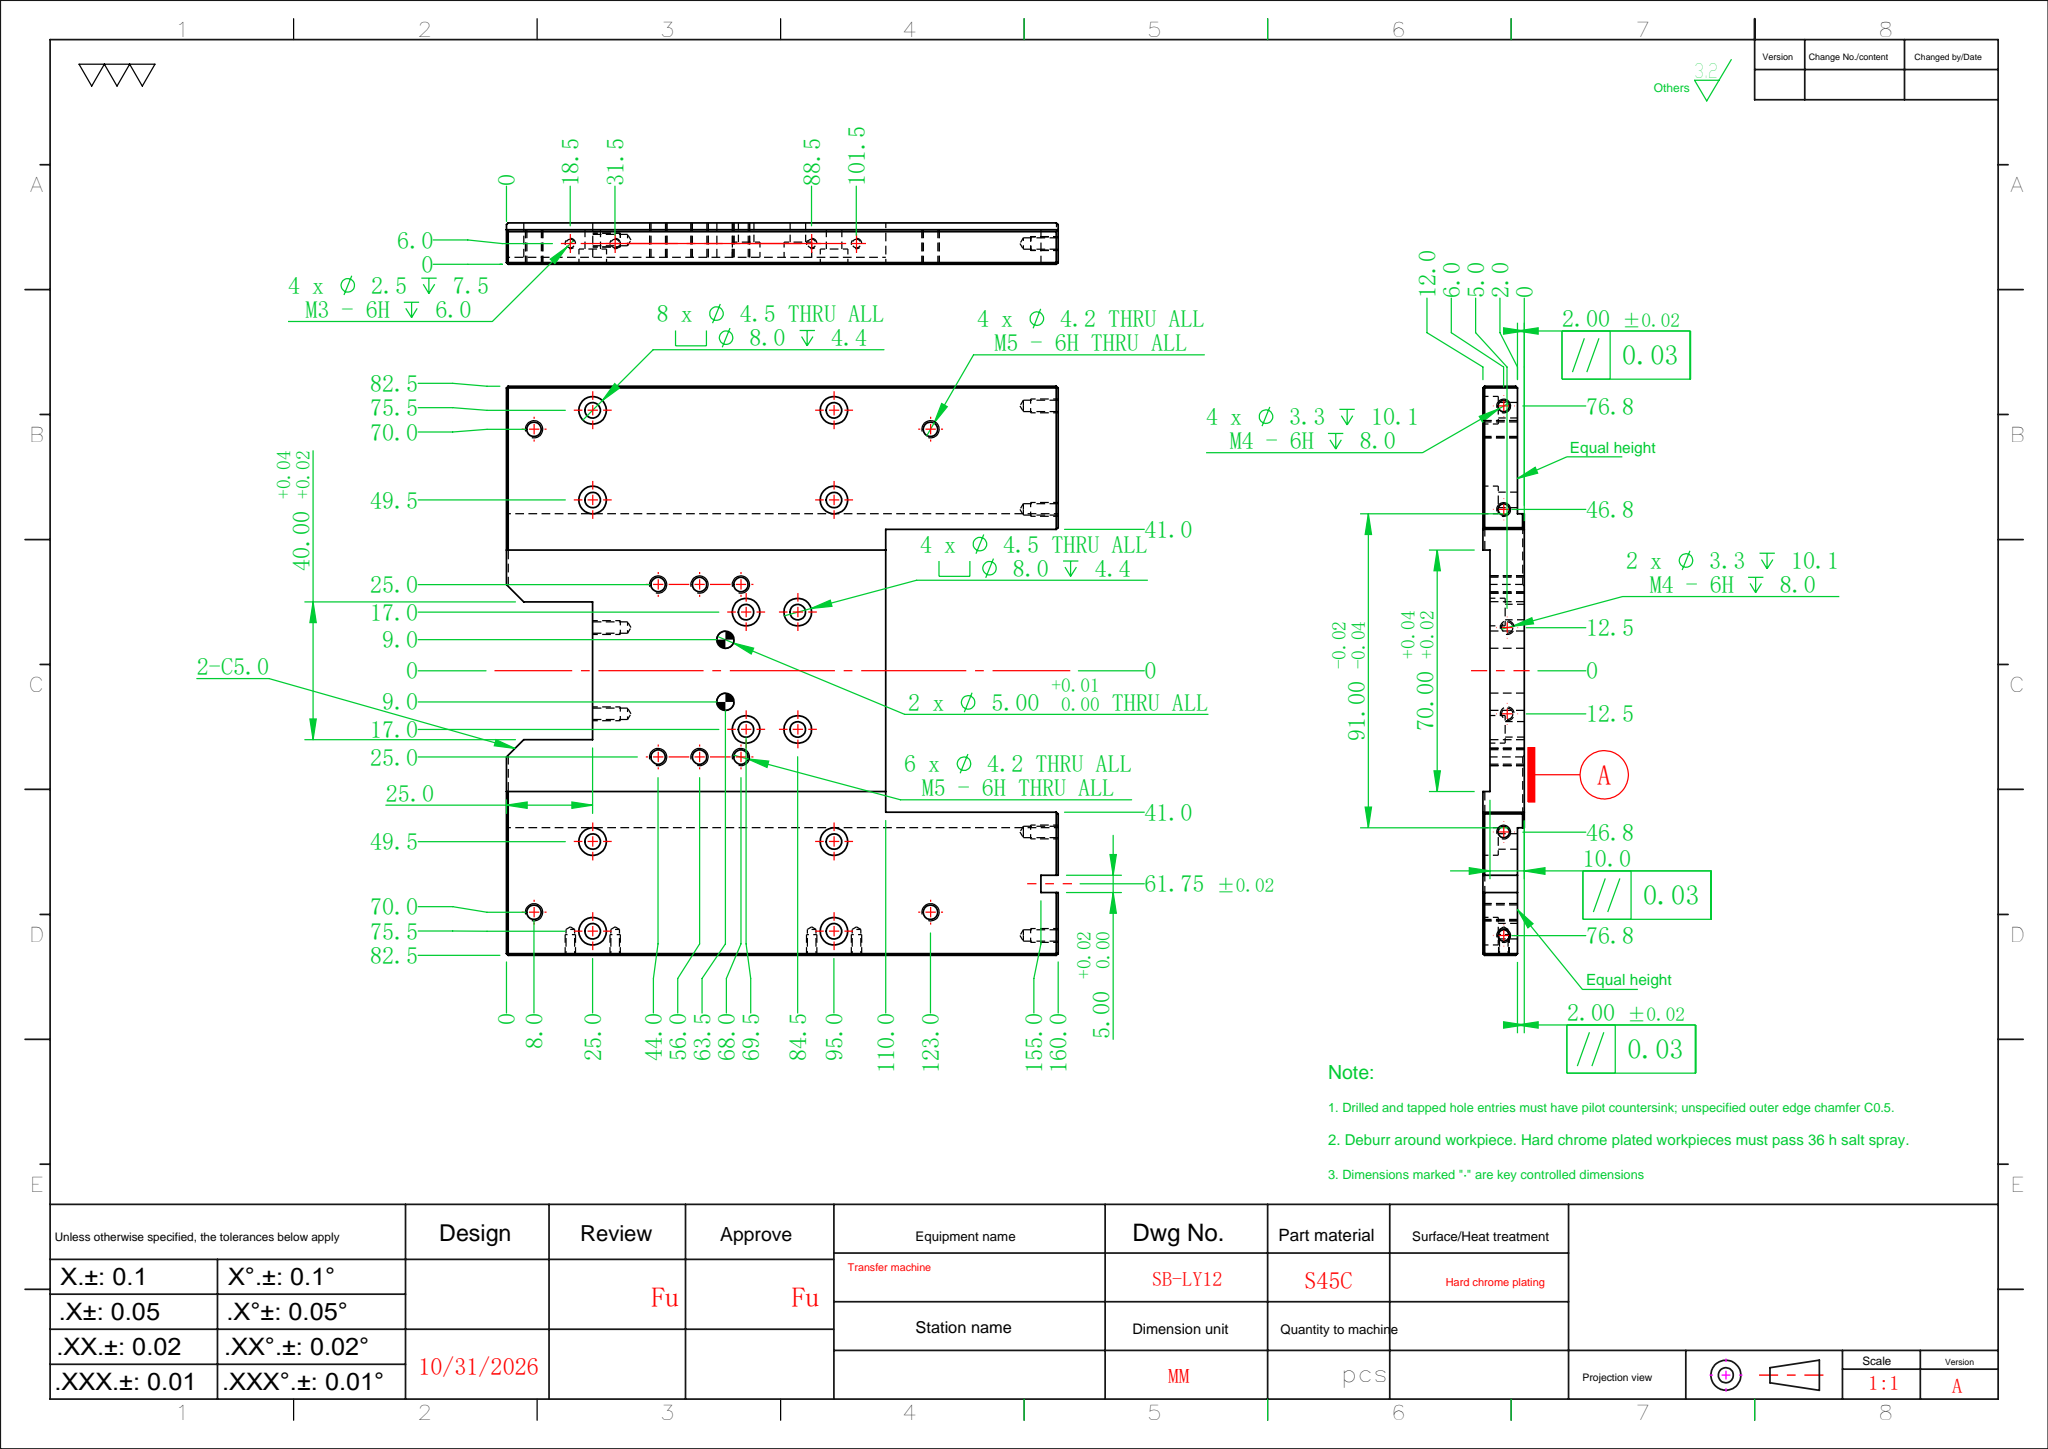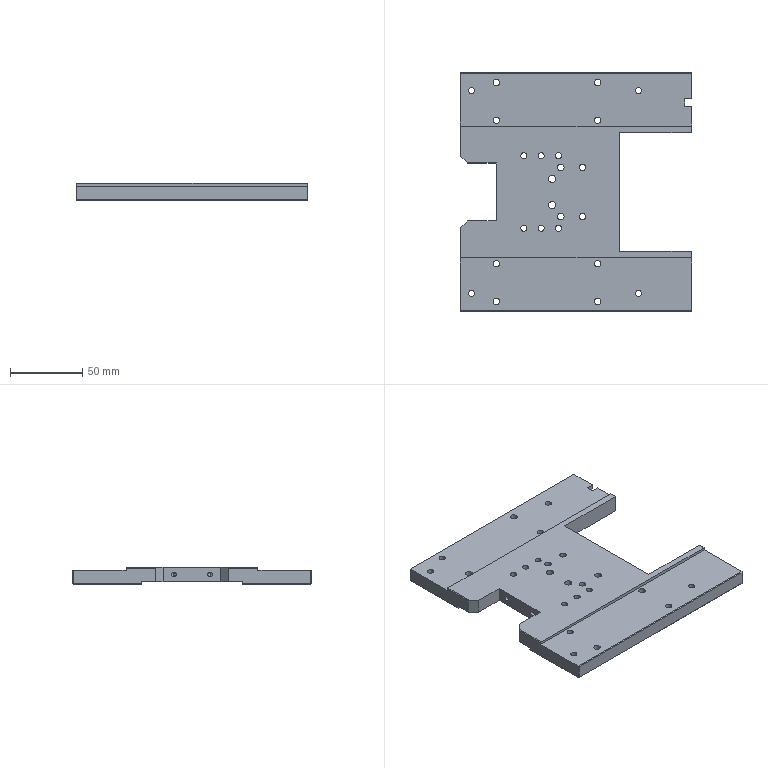Part | SolidWorks | features HoleWzd 8, Cut 4, Chamfer 2, ICE 2, LPattern 2, Extrusion 1 | 1 solid | 175 faces | box 160 x 165 x 12 mm | volume 211716 mm3 | cylinder 92 | plane 63 | cone 20 | commonest cylinder face diameters 4.5 x24 8 x24 4.2 x20 3.3 x12 2.5 x8 5 x4